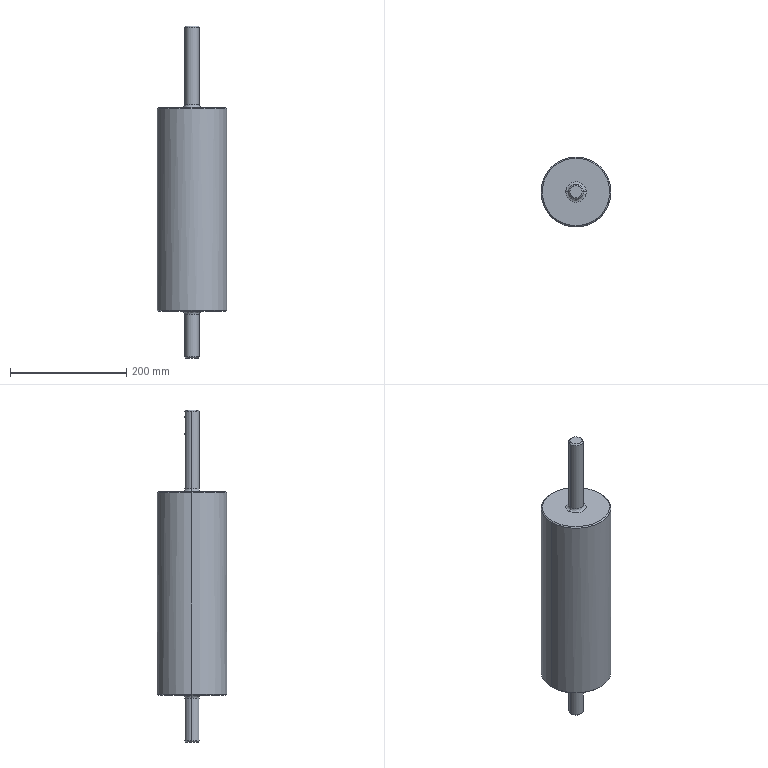Part | STEP file | Roller 1 | 1 solid | 32 faces | box 120 x 120 x 570 mm | volume 928585 mm3 | cylinder 11 | plane 9 | cone 8 | spline 4 | commonest cylinder face diameters 25 x4 8 x3 110 x2 120 x2
STEP:
#1=CARTESIAN_POINT('',(-12.5,0.,-5.));
#2=VERTEX_POINT('',#1);
#3=CARTESIAN_POINT('',(12.5,0.,-5.));
#4=VERTEX_POINT('',#3);
#5=CARTESIAN_POINT('',(0.,0.,-5.));
#6=DIRECTION('',(0.,0.,-1.));
#7=DIRECTION('',(1.,0.,0.));
#8=AXIS2_PLACEMENT_3D('',#5,#6,#7);
#9=CIRCLE('',#8,12.5);
#10=EDGE_CURVE('',#2,#4,#9,.T.);
#11=ORIENTED_EDGE('',*,*,#10,.F.);
#12=CARTESIAN_POINT('',(-17.5,0.,0.));
#13=VERTEX_POINT('',#12);
#14=CARTESIAN_POINT('',(-17.5,0.,-5.));
#15=DIRECTION('',(0.,-1.,0.));
#16=DIRECTION('',(-1.,0.,0.));
#17=AXIS2_PLACEMENT_3D('',#14,#15,#16);
#18=CIRCLE('',#17,5.);
#19=EDGE_CURVE('',#2,#13,#18,.T.);
#20=ORIENTED_EDGE('',*,*,#19,.T.);
#21=CARTESIAN_POINT('',(17.5,0.,0.));
#22=VERTEX_POINT('',#21);
#23=CARTESIAN_POINT('',(-17.5,0.,0.));
#24=CARTESIAN_POINT('',(-17.5,35.,0.));
#25=CARTESIAN_POINT('',(17.5,35.,0.));
#26=CARTESIAN_POINT('',(17.5,0.,0.));
#27=(BOUNDED_CURVE()B_SPLINE_CURVE(3,(#23,#24,#25,#26),.UNSPECIFIED.,.F.,.F.)B_SPLINE_CURVE_WITH_KNOTS((4,4),(0.,1.),.UNSPECIFIED.)CURVE()GEOMETRIC_REPRESENTATION_ITEM()RATIONAL_B_SPLINE_CURVE((1.,0.3333,0.3333,1.))REPRESENTATION_ITEM(''));
#28=EDGE_CURVE('',#13,#22,#27,.T.);
#29=ORIENTED_EDGE('',*,*,#28,.T.);
#30=CARTESIAN_POINT('',(17.5,0.,-5.));
#31=DIRECTION('',(0.,1.,0.));
#32=DIRECTION('',(1.,0.,0.));
#33=AXIS2_PLACEMENT_3D('',#30,#31,#32);
#34=CIRCLE('',#33,5.);
#35=EDGE_CURVE('',#4,#22,#34,.T.);
#36=ORIENTED_EDGE('',*,*,#35,.F.);
#37=EDGE_LOOP('',(#11,#20,#29,#36));
#38=FACE_OUTER_BOUND('',#37,.T.);
#39=CARTESIAN_POINT('',(12.5,0.,-5.));
#40=CARTESIAN_POINT('',(12.5,25.,-5.));
#41=CARTESIAN_POINT('',(-12.5,25.,-5.));
#42=CARTESIAN_POINT('',(-12.5,0.,-5.));
#43=CARTESIAN_POINT('',(12.5,0.,-2.071));
#44=CARTESIAN_POINT('',(12.5,25.,-2.071));
#45=CARTESIAN_POINT('',(-12.5,25.,-2.071));
#46=CARTESIAN_POINT('',(-12.5,0.,-2.071));
#47=CARTESIAN_POINT('',(14.571,0.,0.));
#48=CARTESIAN_POINT('',(14.571,29.142,0.));
#49=CARTESIAN_POINT('',(-14.571,29.142,0.));
#50=CARTESIAN_POINT('',(-14.571,0.,0.));
#51=CARTESIAN_POINT('',(17.5,0.,0.));
#52=CARTESIAN_POINT('',(17.5,35.,0.));
#53=CARTESIAN_POINT('',(-17.5,35.,0.));
#54=CARTESIAN_POINT('',(-17.5,0.,0.));
#55=(BOUNDED_SURFACE()B_SPLINE_SURFACE(3,3,((#39,#40,#41,#42),(#43,#44,#45,#46),(#47,#48,#49,#50),(#51,#52,#53,#54)),.UNSPECIFIED.,.F.,.F.,.F.)B_SPLINE_SURFACE_WITH_KNOTS((4,4),(4,4),(0.,1.),(0.,1.),.UNSPECIFIED.)GEOMETRIC_REPRESENTATION_ITEM()RATIONAL_B_SPLINE_SURFACE(((1.,0.3333,0.3333,1.),(0.8047,0.2682,0.2682,0.8047),(0.8047,0.2682,0.2682,0.8047),(1.,0.3333,0.3333,1.)))REPRESENTATION_ITEM('')SURFACE());
#56=ADVANCED_FACE('',(#38),#55,.F.);
#57=CARTESIAN_POINT('',(-17.5,0.,350.));
#58=VERTEX_POINT('',#57);
#59=CARTESIAN_POINT('',(17.5,0.,350.));
#60=VERTEX_POINT('',#59);
#61=CARTESIAN_POINT('',(-17.5,0.,350.));
#62=CARTESIAN_POINT('',(-17.5,0.5353,350.));
#63=CARTESIAN_POINT('',(-17.463,1.335,350.));
#64=CARTESIAN_POINT('',(-17.357,2.262,350.));
#65=CARTESIAN_POINT('',(-17.288,2.723,350.));
#66=CARTESIAN_POINT('',(-17.249,2.954,350.));
#67=CARTESIAN_POINT('',(-17.232,3.053,350.));
#68=CARTESIAN_POINT('',(-17.22,3.119,350.));
#69=CARTESIAN_POINT('',(-17.214,3.149,350.));
#70=CARTESIAN_POINT('',(-17.105,3.742,350.));
#71=CARTESIAN_POINT('',(-16.91,4.568,350.));
#72=CARTESIAN_POINT('',(-16.614,5.511,350.));
#73=CARTESIAN_POINT('',(-16.448,5.978,350.));
#74=CARTESIAN_POINT('',(-16.361,6.21,350.));
#75=CARTESIAN_POINT('',(-16.323,6.31,350.));
#76=CARTESIAN_POINT('',(-16.297,6.376,350.));
#77=CARTESIAN_POINT('',(-16.285,6.407,350.));
#78=CARTESIAN_POINT('',(-16.054,6.991,350.));
#79=CARTESIAN_POINT('',(-15.688,7.795,350.));
#80=CARTESIAN_POINT('',(-15.191,8.698,350.));
#81=CARTESIAN_POINT('',(-14.925,9.14,350.));
#82=CARTESIAN_POINT('',(-14.807,9.328,350.));
#83=CARTESIAN_POINT('',(-14.728,9.452,350.));
#84=CARTESIAN_POINT('',(-14.689,9.513,350.));
#85=CARTESIAN_POINT('',(-13.987,10.587,350.));
#86=CARTESIAN_POINT('',(-13.228,11.52,350.));
#87=CARTESIAN_POINT('',(-11.947,12.801,350.));
#88=CARTESIAN_POINT('',(-11.277,13.406,350.));
#89=CARTESIAN_POINT('',(-10.444,14.048,350.));
#90=CARTESIAN_POINT('',(-10.014,14.353,350.));
#91=CARTESIAN_POINT('',(-9.828,14.48,350.));
#92=CARTESIAN_POINT('',(-9.702,14.564,350.));
#93=CARTESIAN_POINT('',(-9.638,14.607,350.));
#94=CARTESIAN_POINT('',(-9.081,14.971,350.));
#95=CARTESIAN_POINT('',(-8.318,15.417,350.));
#96=CARTESIAN_POINT('',(-7.392,15.867,350.));
#97=CARTESIAN_POINT('',(-6.92,16.075,350.));
#98=CARTESIAN_POINT('',(-6.682,16.175,350.));
#99=CARTESIAN_POINT('',(-6.579,16.216,350.));
#100=CARTESIAN_POINT('',(-6.51,16.244,350.));
#101=CARTESIAN_POINT('',(-6.475,16.258,350.));
#102=CARTESIAN_POINT('',(-5.914,16.48,350.));
#103=CARTESIAN_POINT('',(-5.111,16.754,350.));
#104=CARTESIAN_POINT('',(-4.155,17.004,350.));
#105=CARTESIAN_POINT('',(-3.671,17.112,350.));
#106=CARTESIAN_POINT('',(-3.428,17.161,350.));
#107=CARTESIAN_POINT('',(-3.324,17.181,350.));
#108=CARTESIAN_POINT('',(-3.254,17.195,350.));
#109=CARTESIAN_POINT('',(-3.217,17.202,350.));
#110=CARTESIAN_POINT('',(-2.132,17.403,350.));
#111=CARTESIAN_POINT('',(-1.07,17.5,350.));
#112=CARTESIAN_POINT('',(0.535,17.5,350.));
#113=CARTESIAN_POINT('',(1.334,17.464,350.));
#114=CARTESIAN_POINT('',(2.261,17.357,350.));
#115=CARTESIAN_POINT('',(2.723,17.288,350.));
#116=CARTESIAN_POINT('',(2.954,17.249,350.));
#117=CARTESIAN_POINT('',(3.053,17.232,350.));
#118=CARTESIAN_POINT('',(3.119,17.22,350.));
#119=CARTESIAN_POINT('',(3.149,17.214,350.));
#120=CARTESIAN_POINT('',(3.742,17.105,350.));
#121=CARTESIAN_POINT('',(4.568,16.91,350.));
#122=CARTESIAN_POINT('',(5.511,16.614,350.));
#123=CARTESIAN_POINT('',(5.978,16.448,350.));
#124=CARTESIAN_POINT('',(6.21,16.361,350.));
#125=CARTESIAN_POINT('',(6.31,16.323,350.));
#126=CARTESIAN_POINT('',(6.376,16.297,350.));
#127=CARTESIAN_POINT('',(6.407,16.285,350.));
#128=CARTESIAN_POINT('',(6.991,16.054,350.));
#129=CARTESIAN_POINT('',(7.795,15.688,350.));
#130=CARTESIAN_POINT('',(8.698,15.191,350.));
#131=CARTESIAN_POINT('',(9.14,14.925,350.));
#132=CARTESIAN_POINT('',(9.328,14.807,350.));
#133=CARTESIAN_POINT('',(9.452,14.728,350.));
#134=CARTESIAN_POINT('',(9.513,14.689,350.));
#135=CARTESIAN_POINT('',(10.587,13.987,350.));
#136=CARTESIAN_POINT('',(11.52,13.228,350.));
#137=CARTESIAN_POINT('',(12.801,11.947,350.));
#138=CARTESIAN_POINT('',(13.406,11.277,350.));
#139=CARTESIAN_POINT('',(14.048,10.444,350.));
#140=CARTESIAN_POINT('',(14.353,10.014,350.));
#141=CARTESIAN_POINT('',(14.48,9.828,350.));
#142=CARTESIAN_POINT('',(14.564,9.702,350.));
#143=CARTESIAN_POINT('',(14.607,9.638,350.));
#144=CARTESIAN_POINT('',(14.971,9.081,350.));
#145=CARTESIAN_POINT('',(15.417,8.318,350.));
#146=CARTESIAN_POINT('',(15.867,7.392,350.));
#147=CARTESIAN_POINT('',(16.075,6.92,350.));
#148=CARTESIAN_POINT('',(16.175,6.682,350.));
#149=CARTESIAN_POINT('',(16.216,6.579,350.));
#150=CARTESIAN_POINT('',(16.244,6.51,350.));
#151=CARTESIAN_POINT('',(16.258,6.475,350.));
#152=CARTESIAN_POINT('',(16.48,5.914,350.));
#153=CARTESIAN_POINT('',(16.754,5.111,350.));
#154=CARTESIAN_POINT('',(17.004,4.155,350.));
#155=CARTESIAN_POINT('',(17.112,3.671,350.));
#156=CARTESIAN_POINT('',(17.161,3.428,350.));
#157=CARTESIAN_POINT('',(17.181,3.324,350.));
#158=CARTESIAN_POINT('',(17.195,3.254,350.));
#159=CARTESIAN_POINT('',(17.202,3.217,350.));
#160=CARTESIAN_POINT('',(17.403,2.132,350.));
#161=CARTESIAN_POINT('',(17.5,1.071,350.));
#162=CARTESIAN_POINT('',(17.5,0.,350.));
#163=B_SPLINE_CURVE_WITH_KNOTS('',3,(#61,#62,#63,#64,#65,#66,#67,#68,#69,#70,#71,#72,#73,#74,#75,#76,#77,#78,#79,#80,#81,#82,#83,#84,#85,#86,#87,#88,#89,#90,#91,#92,#93,#94,#95,#96,#97,#98,#99,#100,#101,#102,#103,#104,#105,#106,#107,#108,#109,#110,#111,#112,#113,#114,#115,#116,#117,#118,#119,#120,#121,#122,#123,#124,#125,#126,#127,#128,#129,#130,#131,#132,#133,#134,#135,#136,#137,#138,#139,#140,#141,#142,#143,#144,#145,#146,#147,#148,#149,#150,#151,#152,#153,#154,#155,#156,#157,#158,#159,#160,#161,#162),.UNSPECIFIED.,.F.,.F.,(4,1,1,1,1,2,2,1,1,1,1,2,2,1,1,1,2,2,2,1,1,1,2,2,1,1,1,1,2,2,1,1,1,1,2,2,2,1,1,1,1,2,2,1,1,1,1,2,2,1,1,1,2,2,2,1,1,1,2,2,1,1,1,1,2,2,1,1,1,1,2,2,4),(0.,0.03125,0.04688,0.05469,0.05859,0.06055,0.0625,0.09375,0.1094,0.1172,0.1211,0.123,0.125,0.1563,0.1719,0.1797,0.1836,0.1875,0.25,0.2813,0.2969,0.3047,0.3086,0.3125,0.3438,0.3594,0.3672,0.3711,0.373,0.375,0.4063,0.4219,0.4297,0.4336,0.4355,0.4375,0.5,0.5313,0.5469,0.5547,0.5586,0.5605,0.5625,0.5938,0.6094,0.6172,0.6211,0.623,0.625,0.6563,0.6719,0.6797,0.6836,0.6875,0.75,0.7813,0.7969,0.8047,0.8086,0.8125,0.8438,0.8594,0.8672,0.8711,0.873,0.875,0.9063,0.9219,0.9297,0.9336,0.9355,0.9375,1.),.UNSPECIFIED.);
#164=EDGE_CURVE('',#58,#60,#163,.T.);
#165=ORIENTED_EDGE('',*,*,#164,.F.);
#166=CARTESIAN_POINT('',(-12.5,0.,355.));
#167=VERTEX_POINT('',#166);
#168=CARTESIAN_POINT('',(-17.5,0.,355.));
#169=DIRECTION('',(0.,-1.,0.));
#170=DIRECTION('',(-1.,0.,0.));
#171=AXIS2_PLACEMENT_3D('',#168,#169,#170);
#172=CIRCLE('',#171,5.);
#173=EDGE_CURVE('',#58,#167,#172,.T.);
#174=ORIENTED_EDGE('',*,*,#173,.T.);
#175=CARTESIAN_POINT('',(12.5,0.,355.));
#176=VERTEX_POINT('',#175);
#177=CARTESIAN_POINT('',(0.,0.,355.));
#178=DIRECTION('',(0.,0.,1.));
#179=DIRECTION('',(1.,0.,0.));
#180=AXIS2_PLACEMENT_3D('',#177,#178,#179);
#181=CIRCLE('',#180,12.5);
#182=EDGE_CURVE('',#176,#167,#181,.T.);
#183=ORIENTED_EDGE('',*,*,#182,.F.);
#184=CARTESIAN_POINT('',(17.5,0.,355.));
#185=DIRECTION('',(0.,1.,0.));
#186=DIRECTION('',(1.,0.,0.));
#187=AXIS2_PLACEMENT_3D('',#184,#185,#186);
#188=CIRCLE('',#187,5.);
#189=EDGE_CURVE('',#60,#176,#188,.T.);
#190=ORIENTED_EDGE('',*,*,#189,.F.);
#191=EDGE_LOOP('',(#165,#174,#183,#190));
#192=FACE_OUTER_BOUND('',#191,.T.);
#193=CARTESIAN_POINT('',(17.5,0.,350.));
#194=CARTESIAN_POINT('',(17.5,35.,350.));
#195=CARTESIAN_POINT('',(-17.5,35.,350.));
#196=CARTESIAN_POINT('',(-17.5,0.,350.));
#197=CARTESIAN_POINT('',(14.571,0.,350.));
#198=CARTESIAN_POINT('',(14.571,29.142,350.));
#199=CARTESIAN_POINT('',(-14.571,29.142,350.));
#200=CARTESIAN_POINT('',(-14.571,0.,350.));
#201=CARTESIAN_POINT('',(12.5,0.,352.071));
#202=CARTESIAN_POINT('',(12.5,25.,352.071));
#203=CARTESIAN_POINT('',(-12.5,25.,352.071));
#204=CARTESIAN_POINT('',(-12.5,0.,352.071));
#205=CARTESIAN_POINT('',(12.5,0.,355.));
#206=CARTESIAN_POINT('',(12.5,25.,355.));
#207=CARTESIAN_POINT('',(-12.5,25.,355.));
#208=CARTESIAN_POINT('',(-12.5,0.,355.));
#209=(BOUNDED_SURFACE()B_SPLINE_SURFACE(3,3,((#193,#194,#195,#196),(#197,#198,#199,#200),(#201,#202,#203,#204),(#205,#206,#207,#208)),.UNSPECIFIED.,.F.,.F.,.F.)B_SPLINE_SURFACE_WITH_KNOTS((4,4),(4,4),(0.,1.),(0.,1.),.UNSPECIFIED.)GEOMETRIC_REPRESENTATION_ITEM()RATIONAL_B_SPLINE_SURFACE(((1.,0.3333,0.3333,1.),(0.8047,0.2682,0.2682,0.8047),(0.8047,0.2682,0.2682,0.8047),(1.,0.3333,0.3333,1.)))REPRESENTATION_ITEM('')SURFACE());
#210=ADVANCED_FACE('',(#192),#209,.F.);
#211=CARTESIAN_POINT('',(0.,60.,348.));
#212=VERTEX_POINT('',#211);
#213=CARTESIAN_POINT('',(60.,0.,348.));
#214=VERTEX_POINT('',#213);
#215=CARTESIAN_POINT('',(0.,0.,348.));
#216=DIRECTION('',(0.,0.,-1.));
#217=DIRECTION('',(-1.,0.,0.));
#218=AXIS2_PLACEMENT_3D('',#215,#216,#217);
#219=CIRCLE('',#218,60.);
#220=EDGE_CURVE('',#212,#214,#219,.T.);
#221=ORIENTED_EDGE('',*,*,#220,.T.);
#222=CARTESIAN_POINT('',(60.,0.,2.));
#223=VERTEX_POINT('',#222);
#224=CARTESIAN_POINT('',(60.,0.,350.));
#225=DIRECTION('',(0.,0.,-1.));
#226=VECTOR('',#225,1000.);
#227=LINE('',#224,#226);
#228=EDGE_CURVE('',#214,#223,#227,.T.);
#229=ORIENTED_EDGE('',*,*,#228,.T.);
#230=CARTESIAN_POINT('',(-60.,0.,2.));
#231=VERTEX_POINT('',#230);
#232=CARTESIAN_POINT('',(0.,0.,2.));
#233=DIRECTION('',(0.,0.,1.));
#234=DIRECTION('',(-1.,0.,0.));
#235=AXIS2_PLACEMENT_3D('',#232,#233,#234);
#236=CIRCLE('',#235,60.);
#237=EDGE_CURVE('',#223,#231,#236,.T.);
#238=ORIENTED_EDGE('',*,*,#237,.T.);
#239=CARTESIAN_POINT('',(-60.,0.,348.));
#240=VERTEX_POINT('',#239);
#241=CARTESIAN_POINT('',(-60.,0.,350.));
#242=DIRECTION('',(0.,0.,-1.));
#243=VECTOR('',#242,1000.);
#244=LINE('',#241,#243);
#245=EDGE_CURVE('',#240,#231,#244,.T.);
#246=ORIENTED_EDGE('',*,*,#245,.F.);
#247=CARTESIAN_POINT('',(0.,0.,348.));
#248=DIRECTION('',(0.,0.,-1.));
#249=DIRECTION('',(-1.,0.,0.));
#250=AXIS2_PLACEMENT_3D('',#247,#248,#249);
#251=CIRCLE('',#250,60.);
#252=EDGE_CURVE('',#240,#212,#251,.T.);
#253=ORIENTED_EDGE('',*,*,#252,.T.);
#254=EDGE_LOOP('',(#221,#229,#238,#246,#253));
#255=FACE_OUTER_BOUND('',#254,.T.);
#256=CARTESIAN_POINT('',(0.,0.,350.));
#257=DIRECTION('',(0.,0.,-1.));
#258=DIRECTION('',(-1.,0.,0.));
#259=AXIS2_PLACEMENT_3D('',#256,#257,#258);
#260=CYLINDRICAL_SURFACE('',#259,60.);
#261=ADVANCED_FACE('',(#255),#260,.T.);
#262=CARTESIAN_POINT('',(58.,0.,0.));
#263=VERTEX_POINT('',#262);
#264=CARTESIAN_POINT('',(-58.,0.,0.));
#265=VERTEX_POINT('',#264);
#266=CARTESIAN_POINT('',(0.,0.,0.));
#267=DIRECTION('',(0.,0.,1.));
#268=DIRECTION('',(1.,0.,0.));
#269=AXIS2_PLACEMENT_3D('',#266,#267,#268);
#270=CIRCLE('',#269,58.);
#271=EDGE_CURVE('',#263,#265,#270,.T.);
#272=ORIENTED_EDGE('',*,*,#271,.T.);
#273=CARTESIAN_POINT('',(-60.,0.,2.));
#274=DIRECTION('',(-0.7071,0.,0.7071));
#275=VECTOR('',#274,1000.);
#276=LINE('',#273,#275);
#277=EDGE_CURVE('',#265,#231,#276,.T.);
#278=ORIENTED_EDGE('',*,*,#277,.T.);
#279=ORIENTED_EDGE('',*,*,#237,.F.);
#280=CARTESIAN_POINT('',(60.,0.,2.));
#281=DIRECTION('',(0.7071,0.,0.7071));
#282=VECTOR('',#281,1000.);
#283=LINE('',#280,#282);
#284=EDGE_CURVE('',#263,#223,#283,.T.);
#285=ORIENTED_EDGE('',*,*,#284,.F.);
#286=EDGE_LOOP('',(#272,#278,#279,#285));
#287=FACE_OUTER_BOUND('',#286,.T.);
#288=CARTESIAN_POINT('',(0.,0.,2.));
#289=DIRECTION('',(0.,0.,1.));
#290=DIRECTION('',(1.,0.,0.));
#291=AXIS2_PLACEMENT_3D('',#288,#289,#290);
#292=CONICAL_SURFACE('',#291,60.,0.7854);
#293=ADVANCED_FACE('',(#287),#292,.T.);
#294=CARTESIAN_POINT('',(0.,58.,350.));
#295=VERTEX_POINT('',#294);
#296=CARTESIAN_POINT('',(0.,-58.,350.));
#297=VERTEX_POINT('',#296);
#298=CARTESIAN_POINT('',(0.,0.,350.));
#299=DIRECTION('',(0.,0.,-1.));
#300=DIRECTION('',(0.,1.,0.));
#301=AXIS2_PLACEMENT_3D('',#298,#299,#300);
#302=CIRCLE('',#301,58.);
#303=EDGE_CURVE('',#295,#297,#302,.T.);
#304=ORIENTED_EDGE('',*,*,#303,.T.);
#305=CARTESIAN_POINT('',(0.,-60.,348.));
#306=VERTEX_POINT('',#305);
#307=CARTESIAN_POINT('',(0.,-60.,348.));
#308=DIRECTION('',(0.,-0.7071,-0.7071));
#309=VECTOR('',#308,1000.);
#310=LINE('',#307,#309);
#311=EDGE_CURVE('',#297,#306,#310,.T.);
#312=ORIENTED_EDGE('',*,*,#311,.T.);
#313=CARTESIAN_POINT('',(0.,0.,348.));
#314=DIRECTION('',(0.,0.,-1.));
#315=DIRECTION('',(-1.,0.,0.));
#316=AXIS2_PLACEMENT_3D('',#313,#314,#315);
#317=CIRCLE('',#316,60.);
#318=EDGE_CURVE('',#214,#306,#317,.T.);
#319=ORIENTED_EDGE('',*,*,#318,.F.);
#320=ORIENTED_EDGE('',*,*,#220,.F.);
#321=CARTESIAN_POINT('',(0.,60.,348.));
#322=DIRECTION('',(0.,0.7071,-0.7071));
#323=VECTOR('',#322,1000.);
#324=LINE('',#321,#323);
#325=EDGE_CURVE('',#295,#212,#324,.T.);
#326=ORIENTED_EDGE('',*,*,#325,.F.);
#327=EDGE_LOOP('',(#304,#312,#319,#320,#326));
#328=FACE_OUTER_BOUND('',#327,.T.);
#329=CARTESIAN_POINT('',(0.,0.,348.));
#330=DIRECTION('',(0.,0.,-1.));
#331=DIRECTION('',(0.,1.,0.));
#332=AXIS2_PLACEMENT_3D('',#329,#330,#331);
#333=CONICAL_SURFACE('',#332,60.,0.7854);
#334=ADVANCED_FACE('',(#328),#333,.T.);
#335=CARTESIAN_POINT('',(12.5,0.,-78.));
#336=VERTEX_POINT('',#335);
#337=CARTESIAN_POINT('',(-12.5,0.,-78.));
#338=VERTEX_POINT('',#337);
#339=CARTESIAN_POINT('',(0.,0.,-78.));
#340=DIRECTION('',(0.,0.,1.));
#341=DIRECTION('',(1.,0.,0.));
#342=AXIS2_PLACEMENT_3D('',#339,#340,#341);
#343=CIRCLE('',#342,12.5);
#344=EDGE_CURVE('',#336,#338,#343,.T.);
#345=ORIENTED_EDGE('',*,*,#344,.T.);
#346=CARTESIAN_POINT('',(-12.5,0.,-80.));
#347=DIRECTION('',(0.,0.,1.));
#348=VECTOR('',#347,1000.);
#349=LINE('',#346,#348);
#350=EDGE_CURVE('',#338,#2,#349,.T.);
#351=ORIENTED_EDGE('',*,*,#350,.T.);
#352=ORIENTED_EDGE('',*,*,#10,.T.);
#353=CARTESIAN_POINT('',(12.5,0.,-80.));
#354=DIRECTION('',(0.,0.,1.));
#355=VECTOR('',#354,1000.);
#356=LINE('',#353,#355);
#357=EDGE_CURVE('',#336,#4,#356,.T.);
#358=ORIENTED_EDGE('',*,*,#357,.F.);
#359=EDGE_LOOP('',(#345,#351,#352,#358));
#360=FACE_OUTER_BOUND('',#359,.T.);
#361=CARTESIAN_POINT('',(0.,0.,-80.));
#362=DIRECTION('',(0.,0.,1.));
#363=DIRECTION('',(1.,0.,0.));
#364=AXIS2_PLACEMENT_3D('',#361,#362,#363);
#365=CYLINDRICAL_SURFACE('',#364,12.5);
#366=ADVANCED_FACE('',(#360),#365,.T.);
#367=CARTESIAN_POINT('',(4.,11.843,452.));
#368=VERTEX_POINT('',#367);
#369=CARTESIAN_POINT('',(4.,11.843,474.));
#370=VERTEX_POINT('',#369);
#371=CARTESIAN_POINT('',(4.,11.843,490.));
#372=DIRECTION('',(0.,0.,1.));
#373=VECTOR('',#372,1000.);
#374=LINE('',#371,#373);
#375=EDGE_CURVE('',#368,#370,#374,.T.);
#376=ORIENTED_EDGE('',*,*,#375,.T.);
#377=CARTESIAN_POINT('',(0.,12.5,478.));
#378=VERTEX_POINT('',#377);
#379=CARTESIAN_POINT('',(4.,11.843,474.));
#380=CARTESIAN_POINT('',(4.,11.843,474.266));
#381=CARTESIAN_POINT('',(3.974,11.852,474.527));
#382=CARTESIAN_POINT('',(3.871,11.886,475.04));
#383=CARTESIAN_POINT('',(3.794,11.911,475.295));
#384=CARTESIAN_POINT('',(3.592,11.973,475.779));
#385=CARTESIAN_POINT('',(3.47,12.01,476.007));
#386=CARTESIAN_POINT('',(3.18,12.09,476.441));
#387=CARTESIAN_POINT('',(3.012,12.133,476.644));
#388=CARTESIAN_POINT('',(2.646,12.218,477.011));
#389=CARTESIAN_POINT('',(2.446,12.26,477.176));
#390=CARTESIAN_POINT('',(2.01,12.339,477.468));
#391=CARTESIAN_POINT('',(1.78,12.375,477.591));
#392=CARTESIAN_POINT('',(1.3,12.435,477.792));
#393=CARTESIAN_POINT('',(1.047,12.459,477.87));
#394=CARTESIAN_POINT('',(0.5285,12.492,477.974));
#395=CARTESIAN_POINT('',(0.266,12.5,478.));
#396=CARTESIAN_POINT('',(0.,12.5,478.));
#397=B_SPLINE_CURVE_WITH_KNOTS('',3,(#379,#380,#381,#382,#383,#384,#385,#386,#387,#388,#389,#390,#391,#392,#393,#394,#395,#396),.UNSPECIFIED.,.F.,.F.,(4,2,2,2,2,2,2,2,4),(-0.00629,-0.005504,-0.004718,-0.003932,-0.003145,-0.002359,-0.001573,-0.0007863,0.),.UNSPECIFIED.);
#398=EDGE_CURVE('',#370,#378,#397,.T.);
#399=ORIENTED_EDGE('',*,*,#398,.T.);
#400=CARTESIAN_POINT('',(-4.,11.843,474.));
#401=VERTEX_POINT('',#400);
#402=CARTESIAN_POINT('',(0.,12.5,478.));
#403=CARTESIAN_POINT('',(-0.266,12.5,478.));
#404=CARTESIAN_POINT('',(-0.5272,12.492,477.974));
#405=CARTESIAN_POINT('',(-1.041,12.459,477.871));
#406=CARTESIAN_POINT('',(-1.296,12.435,477.793));
#407=CARTESIAN_POINT('',(-1.779,12.375,477.592));
#408=CARTESIAN_POINT('',(-2.008,12.34,477.469));
#409=CARTESIAN_POINT('',(-2.441,12.261,477.179));
#410=CARTESIAN_POINT('',(-2.645,12.218,477.012));
#411=CARTESIAN_POINT('',(-3.011,12.133,476.646));
#412=CARTESIAN_POINT('',(-3.176,12.091,476.446));
#413=CARTESIAN_POINT('',(-3.469,12.01,476.009));
#414=CARTESIAN_POINT('',(-3.592,11.973,475.78));
#415=CARTESIAN_POINT('',(-3.792,11.911,475.3));
#416=CARTESIAN_POINT('',(-3.87,11.886,475.046));
#417=CARTESIAN_POINT('',(-3.974,11.852,474.528));
#418=CARTESIAN_POINT('',(-4.,11.843,474.266));
#419=CARTESIAN_POINT('',(-4.,11.843,474.));
#420=B_SPLINE_CURVE_WITH_KNOTS('',3,(#402,#403,#404,#405,#406,#407,#408,#409,#410,#411,#412,#413,#414,#415,#416,#417,#418,#419),.UNSPECIFIED.,.F.,.F.,(4,2,2,2,2,2,2,2,4),(0.,0.0007863,0.001573,0.002359,0.003145,0.003932,0.004718,0.005504,0.00629),.UNSPECIFIED.);
#421=EDGE_CURVE('',#378,#401,#420,.T.);
#422=ORIENTED_EDGE('',*,*,#421,.T.);
#423=CARTESIAN_POINT('',(-4.,11.843,452.));
#424=VERTEX_POINT('',#423);
#425=CARTESIAN_POINT('',(-4.,11.843,490.));
#426=DIRECTION('',(0.,0.,-1.));
#427=VECTOR('',#426,1000.);
#428=LINE('',#425,#427);
#429=EDGE_CURVE('',#401,#424,#428,.T.);
#430=ORIENTED_EDGE('',*,*,#429,.T.);
#431=CARTESIAN_POINT('',(-4.,11.843,452.));
#432=CARTESIAN_POINT('',(-4.,11.843,451.734));
#433=CARTESIAN_POINT('',(-3.974,11.852,451.473));
#434=CARTESIAN_POINT('',(-3.871,11.886,450.959));
#435=CARTESIAN_POINT('',(-3.793,11.911,450.704));
#436=CARTESIAN_POINT('',(-3.592,11.973,450.221));
#437=CARTESIAN_POINT('',(-3.469,12.01,449.992));
#438=CARTESIAN_POINT('',(-3.179,12.09,449.559));
#439=CARTESIAN_POINT('',(-3.012,12.133,449.355));
#440=CARTESIAN_POINT('',(-2.646,12.218,448.989));
#441=CARTESIAN_POINT('',(-2.445,12.26,448.824));
#442=CARTESIAN_POINT('',(-2.009,12.34,448.531));
#443=CARTESIAN_POINT('',(-1.779,12.375,448.408));
#444=CARTESIAN_POINT('',(-1.299,12.435,448.208));
#445=CARTESIAN_POINT('',(-1.045,12.459,448.13));
#446=CARTESIAN_POINT('',(-0.5276,12.492,448.026));
#447=CARTESIAN_POINT('',(-0.2669,12.5,448.));
#448=CARTESIAN_POINT('',(0.2587,12.5,448.));
#449=CARTESIAN_POINT('',(0.5256,12.492,448.026));
#450=CARTESIAN_POINT('',(1.04,12.459,448.129));
#451=CARTESIAN_POINT('',(1.29,12.436,448.205));
#452=CARTESIAN_POINT('',(1.777,12.375,448.407));
#453=CARTESIAN_POINT('',(2.008,12.34,448.531));
#454=CARTESIAN_POINT('',(2.44,12.262,448.82));
#455=CARTESIAN_POINT('',(2.643,12.219,448.987));
#456=CARTESIAN_POINT('',(3.012,12.133,449.355));
#457=CARTESIAN_POINT('',(3.176,12.091,449.555));
#458=CARTESIAN_POINT('',(3.466,12.011,449.987));
#459=CARTESIAN_POINT('',(3.592,11.973,450.22));
#460=CARTESIAN_POINT('',(3.792,11.911,450.702));
#461=CARTESIAN_POINT('',(3.869,11.886,450.951));
#462=CARTESIAN_POINT('',(3.973,11.852,451.468));
#463=CARTESIAN_POINT('',(4.,11.843,451.734));
#464=CARTESIAN_POINT('',(4.,11.843,452.));
#465=B_SPLINE_CURVE_WITH_KNOTS('',3,(#431,#432,#433,#434,#435,#436,#437,#438,#439,#440,#441,#442,#443,#444,#445,#446,#447,#448,#449,#450,#451,#452,#453,#454,#455,#456,#457,#458,#459,#460,#461,#462,#463,#464),.UNSPECIFIED.,.F.,.F.,(4,2,2,2,2,2,2,2,2,2,2,2,2,2,2,2,4),(0.,0.0007865,0.001573,0.00236,0.003146,0.003933,0.004719,0.005506,0.006292,0.007079,0.007865,0.008652,0.009438,0.01022,0.01101,0.0118,0.01258),.UNSPECIFIED.);
#466=EDGE_CURVE('',#424,#368,#465,.T.);
#467=ORIENTED_EDGE('',*,*,#466,.T.);
#468=EDGE_LOOP('',(#376,#399,#422,#430,#467));
#469=FACE_BOUND('',#468,.T.);
#470=CARTESIAN_POINT('',(-12.5,0.,488.));
#471=VERTEX_POINT('',#470);
#472=CARTESIAN_POINT('',(12.5,0.,488.));
#473=VERTEX_POINT('',#472);
#474=CARTESIAN_POINT('',(0.,0.,488.));
#475=DIRECTION('',(0.,0.,-1.));
#476=DIRECTION('',(-1.,0.,0.));
#477=AXIS2_PLACEMENT_3D('',#474,#475,#476);
#478=CIRCLE('',#477,12.5);
#479=EDGE_CURVE('',#471,#473,#478,.T.);
#480=ORIENTED_EDGE('',*,*,#479,.T.);
#481=CARTESIAN_POINT('',(12.5,0.,490.));
#482=DIRECTION('',(0.,0.,-1.));
#483=VECTOR('',#482,1000.);
#484=LINE('',#481,#483);
#485=EDGE_CURVE('',#473,#176,#484,.T.);
#486=ORIENTED_EDGE('',*,*,#485,.T.);
#487=ORIENTED_EDGE('',*,*,#182,.T.);
#488=CARTESIAN_POINT('',(-12.5,0.,490.));
#489=DIRECTION('',(0.,0.,-1.));
#490=VECTOR('',#489,1000.);
#491=LINE('',#488,#490);
#492=EDGE_CURVE('',#471,#167,#491,.T.);
#493=ORIENTED_EDGE('',*,*,#492,.F.);
#494=EDGE_LOOP('',(#480,#486,#487,#493));
#495=FACE_OUTER_BOUND('',#494,.T.);
#496=CARTESIAN_POINT('',(0.,0.,490.));
#497=DIRECTION('',(0.,0.,-1.));
#498=DIRECTION('',(-1.,0.,0.));
#499=AXIS2_PLACEMENT_3D('',#496,#497,#498);
#500=CYLINDRICAL_SURFACE('',#499,12.5);
#501=ADVANCED_FACE('',(#469,#495),#500,.T.);
#502=CARTESIAN_POINT('',(10.5,0.,-80.));
#503=VERTEX_POINT('',#502);
#504=CARTESIAN_POINT('',(-10.5,0.,-80.));
#505=VERTEX_POINT('',#504);
#506=CARTESIAN_POINT('',(0.,0.,-80.));
#507=DIRECTION('',(0.,0.,1.));
#508=DIRECTION('',(1.,0.,0.));
#509=AXIS2_PLACEMENT_3D('',#506,#507,#508);
#510=CIRCLE('',#509,10.5);
#511=EDGE_CURVE('',#503,#505,#510,.T.);
#512=ORIENTED_EDGE('',*,*,#511,.T.);
#513=CARTESIAN_POINT('',(-12.5,0.,-78.));
#514=DIRECTION('',(-0.7071,0.,0.7071));
#515=VECTOR('',#514,1000.);
#516=LINE('',#513,#515);
#517=EDGE_CURVE('',#505,#338,#516,.T.);
#518=ORIENTED_EDGE('',*,*,#517,.T.);
#519=ORIENTED_EDGE('',*,*,#344,.F.);
#520=CARTESIAN_POINT('',(12.5,0.,-78.));
#521=DIRECTION('',(0.7071,0.,0.7071));
#522=VECTOR('',#521,1000.);
#523=LINE('',#520,#522);
#524=EDGE_CURVE('',#503,#336,#523,.T.);
#525=ORIENTED_EDGE('',*,*,#524,.F.);
#526=EDGE_LOOP('',(#512,#518,#519,#525));
#527=FACE_OUTER_BOUND('',#526,.T.);
#528=CARTESIAN_POINT('',(0.,0.,-78.));
#529=DIRECTION('',(0.,0.,1.));
#530=DIRECTION('',(1.,0.,0.));
#531=AXIS2_PLACEMENT_3D('',#528,#529,#530);
#532=CONICAL_SURFACE('',#531,12.5,0.7854);
#533=ADVANCED_FACE('',(#527),#532,.T.);
#534=CARTESIAN_POINT('',(-10.5,0.,490.));
#535=VERTEX_POINT('',#534);
#536=CARTESIAN_POINT('',(10.5,0.,490.));
#537=VERTEX_POINT('',#536);
#538=CARTESIAN_POINT('',(0.,0.,490.));
#539=DIRECTION('',(0.,0.,-1.));
#540=DIRECTION('',(-1.,0.,0.));
#541=AXIS2_PLACEMENT_3D('',#538,#539,#540);
#542=CIRCLE('',#541,10.5);
#543=EDGE_CURVE('',#535,#537,#542,.T.);
#544=ORIENTED_EDGE('',*,*,#543,.T.);
#545=CARTESIAN_POINT('',(12.5,0.,488.));
#546=DIRECTION('',(0.7071,0.,-0.7071));
#547=VECTOR('',#546,1000.);
#548=LINE('',#545,#547);
#549=EDGE_CURVE('',#537,#473,#548,.T.);
#550=ORIENTED_EDGE('',*,*,#549,.T.);
#551=ORIENTED_EDGE('',*,*,#479,.F.);
#552=CARTESIAN_POINT('',(-12.5,0.,488.));
#553=DIRECTION('',(-0.7071,0.,-0.7071));
#554=VECTOR('',#553,1000.);
#555=LINE('',#552,#554);
#556=EDGE_CURVE('',#535,#471,#555,.T.);
#557=ORIENTED_EDGE('',*,*,#556,.F.);
#558=EDGE_LOOP('',(#544,#550,#551,#557));
#559=FACE_OUTER_BOUND('',#558,.T.);
#560=CARTESIAN_POINT('',(0.,0.,488.));
#561=DIRECTION('',(0.,0.,-1.));
#562=DIRECTION('',(-1.,0.,0.));
#563=AXIS2_PLACEMENT_3D('',#560,#561,#562);
#564=CONICAL_SURFACE('',#563,12.5,0.7854);
#565=ADVANCED_FACE('',(#559),#564,.T.);
#566=CARTESIAN_POINT('',(0.,8.5,478.));
#567=VERTEX_POINT('',#566);
#568=CARTESIAN_POINT('',(4.,8.5,474.));
#569=VERTEX_POINT('',#568);
#570=CARTESIAN_POINT('',(0.,8.5,474.));
#571=DIRECTION('',(0.,1.,0.));
#572=DIRECTION('',(0.,0.,1.));
#573=AXIS2_PLACEMENT_3D('',#570,#571,#572);
#574=CIRCLE('',#573,4.);
#575=EDGE_CURVE('',#567,#569,#574,.T.);
#576=ORIENTED_EDGE('',*,*,#575,.F.);
#577=CARTESIAN_POINT('',(0.,8.5,478.));
#578=DIRECTION('',(0.,1.,0.));
#579=VECTOR('',#578,1000.);
#580=LINE('',#577,#579);
#581=EDGE_CURVE('',#567,#378,#580,.T.);
#582=ORIENTED_EDGE('',*,*,#581,.T.);
#583=ORIENTED_EDGE('',*,*,#398,.F.);
#584=CARTESIAN_POINT('',(4.,8.5,474.));
#585=DIRECTION('',(0.,1.,0.));
#586=VECTOR('',#585,1000.);
#587=LINE('',#584,#586);
#588=EDGE_CURVE('',#569,#370,#587,.T.);
#589=ORIENTED_EDGE('',*,*,#588,.F.);
#590=EDGE_LOOP('',(#576,#582,#583,#589));
#591=FACE_OUTER_BOUND('',#590,.T.);
#592=CARTESIAN_POINT('',(0.,8.5,474.));
#593=DIRECTION('',(0.,1.,0.));
#594=DIRECTION('',(0.,0.,1.));
#595=AXIS2_PLACEMENT_3D('',#592,#593,#594);
#596=CYLINDRICAL_SURFACE('',#595,4.);
#597=ADVANCED_FACE('',(#591),#596,.F.);
#598=CARTESIAN_POINT('',(4.,8.5,452.));
#599=VERTEX_POINT('',#598);
#600=CARTESIAN_POINT('',(-4.,8.5,452.));
#601=VERTEX_POINT('',#600);
#602=CARTESIAN_POINT('',(0.,8.5,452.));
#603=DIRECTION('',(0.,1.,0.));
#604=DIRECTION('',(0.,0.,1.));
#605=AXIS2_PLACEMENT_3D('',#602,#603,#604);
#606=CIRCLE('',#605,4.);
#607=EDGE_CURVE('',#599,#601,#606,.T.);
#608=ORIENTED_EDGE('',*,*,#607,.T.);
#609=CARTESIAN_POINT('',(-4.,8.5,474.));
#610=VERTEX_POINT('',#609);
#611=CARTESIAN_POINT('',(-4.,8.5,474.));
#612=DIRECTION('',(0.,0.,1.));
#613=VECTOR('',#612,1000.);
#614=LINE('',#611,#613);
#615=EDGE_CURVE('',#601,#610,#614,.T.);
#616=ORIENTED_EDGE('',*,*,#615,.T.);
#617=CARTESIAN_POINT('',(0.,8.5,474.));
#618=DIRECTION('',(0.,1.,0.));
#619=DIRECTION('',(0.,0.,1.));
#620=AXIS2_PLACEMENT_3D('',#617,#618,#619);
#621=CIRCLE('',#620,4.);
#622=EDGE_CURVE('',#610,#567,#621,.T.);
#623=ORIENTED_EDGE('',*,*,#622,.T.);
#624=ORIENTED_EDGE('',*,*,#575,.T.);
#625=CARTESIAN_POINT('',(4.,8.5,474.));
#626=DIRECTION('',(0.,0.,-1.));
#627=VECTOR('',#626,1000.);
#628=LINE('',#625,#627);
#629=EDGE_CURVE('',#569,#599,#628,.T.);
#630=ORIENTED_EDGE('',*,*,#629,.T.);
#631=EDGE_LOOP('',(#608,#616,#623,#624,#630));
#632=FACE_OUTER_BOUND('',#631,.T.);
#633=CARTESIAN_POINT('',(0.,8.5,474.));
#634=DIRECTION('',(0.,1.,0.));
#635=DIRECTION('',(0.,0.,1.));
#636=AXIS2_PLACEMENT_3D('',#633,#634,#635);
#637=PLANE('',#636);
#638=ADVANCED_FACE('',(#632),#637,.T.);
#639=ORIENTED_EDGE('',*,*,#543,.F.);
#640=CARTESIAN_POINT('',(0.,0.,490.));
#641=DIRECTION('',(0.,0.,-1.));
#642=DIRECTION('',(-1.,0.,0.));
#643=AXIS2_PLACEMENT_3D('',#640,#641,#642);
#644=CIRCLE('',#643,10.5);
#645=EDGE_CURVE('',#537,#535,#644,.T.);
#646=ORIENTED_EDGE('',*,*,#645,.F.);
#647=EDGE_LOOP('',(#639,#646));
#648=FACE_OUTER_BOUND('',#647,.T.);
#649=CARTESIAN_POINT('',(0.,0.,490.));
#650=DIRECTION('',(0.,0.,1.));
#651=DIRECTION('',(1.,0.,0.));
#652=AXIS2_PLACEMENT_3D('',#649,#650,#651);
#653=PLANE('',#652);
#654=ADVANCED_FACE('',(#648),#653,.T.);
#655=ORIENTED_EDGE('',*,*,#511,.F.);
#656=CARTESIAN_POINT('',(0.,0.,-80.));
#657=DIRECTION('',(0.,0.,1.));
#658=DIRECTION('',(1.,0.,0.));
#659=AXIS2_PLACEMENT_3D('',#656,#657,#658);
#660=CIRCLE('',#659,10.5);
#661=EDGE_CURVE('',#505,#503,#660,.T.);
#662=ORIENTED_EDGE('',*,*,#661,.F.);
#663=EDGE_LOOP('',(#655,#662));
#664=FACE_OUTER_BOUND('',#663,.T.);
#665=CARTESIAN_POINT('',(0.,0.,-80.));
#666=DIRECTION('',(0.,0.,-1.));
#667=DIRECTION('',(-1.,0.,0.));
#668=AXIS2_PLACEMENT_3D('',#665,#666,#667);
#669=PLANE('',#668);
#670=ADVANCED_FACE('',(#664),#669,.T.);
#671=ORIENTED_EDGE('',*,*,#615,.F.);
#672=CARTESIAN_POINT('',(-4.,8.5,452.));
#673=DIRECTION('',(0.,1.,0.));
#674=VECTOR('',#673,1000.);
#675=LINE('',#672,#674);
#676=EDGE_CURVE('',#601,#424,#675,.T.);
#677=ORIENTED_EDGE('',*,*,#676,.T.);
#678=ORIENTED_EDGE('',*,*,#429,.F.);
#679=CARTESIAN_POINT('',(-4.,8.5,474.));
#680=DIRECTION('',(0.,-1.,0.));
#681=VECTOR('',#680,1000.);
#682=LINE('',#679,#681);
#683=EDGE_CURVE('',#401,#610,#682,.T.);
#684=ORIENTED_EDGE('',*,*,#683,.T.);
#685=EDGE_LOOP('',(#671,#677,#678,#684));
#686=FACE_OUTER_BOUND('',#685,.T.);
#687=CARTESIAN_POINT('',(-4.,8.5,474.));
#688=DIRECTION('',(-1.,0.,0.));
#689=DIRECTION('',(0.,0.,1.));
#690=AXIS2_PLACEMENT_3D('',#687,#688,#689);
#691=PLANE('',#690);
#692=ADVANCED_FACE('',(#686),#691,.F.);
#693=ORIENTED_EDGE('',*,*,#607,.F.);
#694=CARTESIAN_POINT('',(4.,8.5,452.));
#695=DIRECTION('',(0.,1.,0.));
#696=VECTOR('',#695,1000.);
#697=LINE('',#694,#696);
#698=EDGE_CURVE('',#599,#368,#697,.T.);
#699=ORIENTED_EDGE('',*,*,#698,.T.);
#700=ORIENTED_EDGE('',*,*,#466,.F.);
#701=ORIENTED_EDGE('',*,*,#676,.F.);
#702=EDGE_LOOP('',(#693,#699,#700,#701));
#703=FACE_OUTER_BOUND('',#702,.T.);
#704=CARTESIAN_POINT('',(0.,8.5,452.));
#705=DIRECTION('',(0.,1.,0.));
#706=DIRECTION('',(0.,0.,1.));
#707=AXIS2_PLACEMENT_3D('',#704,#705,#706);
#708=CYLINDRICAL_SURFACE('',#707,4.);
#709=ADVANCED_FACE('',(#703),#708,.F.);
#710=ORIENTED_EDGE('',*,*,#629,.F.);
#711=ORIENTED_EDGE('',*,*,#588,.T.);
#712=ORIENTED_EDGE('',*,*,#375,.F.);
#713=ORIENTED_EDGE('',*,*,#698,.F.);
#714=EDGE_LOOP('',(#710,#711,#712,#713));
#715=FACE_OUTER_BOUND('',#714,.T.);
#716=CARTESIAN_POINT('',(4.,8.5,474.));
#717=DIRECTION('',(1.,0.,0.));
#718=DIRECTION('',(0.,0.,-1.));
#719=AXIS2_PLACEMENT_3D('',#716,#717,#718);
#720=PLANE('',#719);
#721=ADVANCED_FACE('',(#715),#720,.F.);
#722=ORIENTED_EDGE('',*,*,#581,.F.);
#723=ORIENTED_EDGE('',*,*,#622,.F.);
#724=ORIENTED_EDGE('',*,*,#683,.F.);
#725=ORIENTED_EDGE('',*,*,#421,.F.);
#726=EDGE_LOOP('',(#722,#723,#724,#725));
#727=FACE_OUTER_BOUND('',#726,.T.);
#728=CARTESIAN_POINT('',(0.,8.5,474.));
#729=DIRECTION('',(0.,1.,0.));
#730=DIRECTION('',(0.,0.,1.));
#731=AXIS2_PLACEMENT_3D('',#728,#729,#730);
#732=CYLINDRICAL_SURFACE('',#731,4.);
#733=ADVANCED_FACE('',(#727),#732,.F.);
#734=ORIENTED_EDGE('',*,*,#549,.F.);
#735=ORIENTED_EDGE('',*,*,#645,.T.);
#736=ORIENTED_EDGE('',*,*,#556,.T.);
#737=CARTESIAN_POINT('',(0.,0.,488.));
#738=DIRECTION('',(0.,0.,-1.));
#739=DIRECTION('',(-1.,0.,0.));
#740=AXIS2_PLACEMENT_3D('',#737,#738,#739);
#741=CIRCLE('',#740,12.5);
#742=EDGE_CURVE('',#473,#471,#741,.T.);
#743=ORIENTED_EDGE('',*,*,#742,.F.);
#744=EDGE_LOOP('',(#734,#735,#736,#743));
#745=FACE_OUTER_BOUND('',#744,.T.);
#746=CARTESIAN_POINT('',(0.,0.,488.));
#747=DIRECTION('',(0.,0.,-1.));
#748=DIRECTION('',(-1.,0.,0.));
#749=AXIS2_PLACEMENT_3D('',#746,#747,#748);
#750=CONICAL_SURFACE('',#749,12.5,0.7854);
#751=ADVANCED_FACE('',(#745),#750,.T.);
#752=ORIENTED_EDGE('',*,*,#517,.F.);
#753=ORIENTED_EDGE('',*,*,#661,.T.);
#754=ORIENTED_EDGE('',*,*,#524,.T.);
#755=CARTESIAN_POINT('',(0.,0.,-78.));
#756=DIRECTION('',(0.,0.,1.));
#757=DIRECTION('',(1.,0.,0.));
#758=AXIS2_PLACEMENT_3D('',#755,#756,#757);
#759=CIRCLE('',#758,12.5);
#760=EDGE_CURVE('',#338,#336,#759,.T.);
#761=ORIENTED_EDGE('',*,*,#760,.F.);
#762=EDGE_LOOP('',(#752,#753,#754,#761));
#763=FACE_OUTER_BOUND('',#762,.T.);
#764=CARTESIAN_POINT('',(0.,0.,-78.));
#765=DIRECTION('',(0.,0.,1.));
#766=DIRECTION('',(1.,0.,0.));
#767=AXIS2_PLACEMENT_3D('',#764,#765,#766);
#768=CONICAL_SURFACE('',#767,12.5,0.7854);
#769=ADVANCED_FACE('',(#763),#768,.T.);
#770=ORIENTED_EDGE('',*,*,#485,.F.);
#771=ORIENTED_EDGE('',*,*,#742,.T.);
#772=ORIENTED_EDGE('',*,*,#492,.T.);
#773=CARTESIAN_POINT('',(0.,0.,355.));
#774=DIRECTION('',(0.,0.,1.));
#775=DIRECTION('',(1.,0.,0.));
#776=AXIS2_PLACEMENT_3D('',#773,#774,#775);
#777=CIRCLE('',#776,12.5);
#778=EDGE_CURVE('',#167,#176,#777,.T.);
#779=ORIENTED_EDGE('',*,*,#778,.T.);
#780=EDGE_LOOP('',(#770,#771,#772,#779));
#781=FACE_OUTER_BOUND('',#780,.T.);
#782=CARTESIAN_POINT('',(0.,0.,490.));
#783=DIRECTION('',(0.,0.,-1.));
#784=DIRECTION('',(-1.,0.,0.));
#785=AXIS2_PLACEMENT_3D('',#782,#783,#784);
#786=CYLINDRICAL_SURFACE('',#785,12.5);
#787=ADVANCED_FACE('',(#781),#786,.T.);
#788=ORIENTED_EDGE('',*,*,#350,.F.);
#789=ORIENTED_EDGE('',*,*,#760,.T.);
#790=ORIENTED_EDGE('',*,*,#357,.T.);
#791=CARTESIAN_POINT('',(0.,0.,-5.));
#792=DIRECTION('',(0.,0.,-1.));
#793=DIRECTION('',(1.,0.,0.));
#794=AXIS2_PLACEMENT_3D('',#791,#792,#793);
#795=CIRCLE('',#794,12.5);
#796=EDGE_CURVE('',#4,#2,#795,.T.);
#797=ORIENTED_EDGE('',*,*,#796,.T.);
#798=EDGE_LOOP('',(#788,#789,#790,#797));
#799=FACE_OUTER_BOUND('',#798,.T.);
#800=CARTESIAN_POINT('',(0.,0.,-80.));
#801=DIRECTION('',(0.,0.,1.));
#802=DIRECTION('',(1.,0.,0.));
#803=AXIS2_PLACEMENT_3D('',#800,#801,#802);
#804=CYLINDRICAL_SURFACE('',#803,12.5);
#805=ADVANCED_FACE('',(#799),#804,.T.);
#806=ORIENTED_EDGE('',*,*,#173,.F.);
#807=CARTESIAN_POINT('',(17.5,0.,350.));
#808=CARTESIAN_POINT('',(17.5,-0.5353,350.));
#809=CARTESIAN_POINT('',(17.463,-1.335,350.));
#810=CARTESIAN_POINT('',(17.357,-2.262,350.));
#811=CARTESIAN_POINT('',(17.288,-2.723,350.));
#812=CARTESIAN_POINT('',(17.249,-2.954,350.));
#813=CARTESIAN_POINT('',(17.232,-3.053,350.));
#814=CARTESIAN_POINT('',(17.22,-3.119,350.));
#815=CARTESIAN_POINT('',(17.214,-3.149,350.));
#816=CARTESIAN_POINT('',(17.105,-3.742,350.));
#817=CARTESIAN_POINT('',(16.91,-4.568,350.));
#818=CARTESIAN_POINT('',(16.614,-5.511,350.));
#819=CARTESIAN_POINT('',(16.448,-5.978,350.));
#820=CARTESIAN_POINT('',(16.361,-6.21,350.));
#821=CARTESIAN_POINT('',(16.323,-6.31,350.));
#822=CARTESIAN_POINT('',(16.297,-6.376,350.));
#823=CARTESIAN_POINT('',(16.285,-6.407,350.));
#824=CARTESIAN_POINT('',(16.054,-6.991,350.));
#825=CARTESIAN_POINT('',(15.688,-7.795,350.));
#826=CARTESIAN_POINT('',(15.191,-8.698,350.));
#827=CARTESIAN_POINT('',(14.925,-9.14,350.));
#828=CARTESIAN_POINT('',(14.807,-9.328,350.));
#829=CARTESIAN_POINT('',(14.728,-9.452,350.));
#830=CARTESIAN_POINT('',(14.689,-9.513,350.));
#831=CARTESIAN_POINT('',(13.987,-10.587,350.));
#832=CARTESIAN_POINT('',(13.228,-11.52,350.));
#833=CARTESIAN_POINT('',(11.947,-12.801,350.));
#834=CARTESIAN_POINT('',(11.277,-13.406,350.));
#835=CARTESIAN_POINT('',(10.444,-14.048,350.));
#836=CARTESIAN_POINT('',(10.014,-14.353,350.));
#837=CARTESIAN_POINT('',(9.828,-14.48,350.));
#838=CARTESIAN_POINT('',(9.702,-14.564,350.));
#839=CARTESIAN_POINT('',(9.638,-14.607,350.));
#840=CARTESIAN_POINT('',(9.081,-14.971,350.));
#841=CARTESIAN_POINT('',(8.318,-15.417,350.));
#842=CARTESIAN_POINT('',(7.392,-15.867,350.));
#843=CARTESIAN_POINT('',(6.92,-16.075,350.));
#844=CARTESIAN_POINT('',(6.682,-16.175,350.));
#845=CARTESIAN_POINT('',(6.579,-16.216,350.));
#846=CARTESIAN_POINT('',(6.51,-16.244,350.));
#847=CARTESIAN_POINT('',(6.475,-16.258,350.));
#848=CARTESIAN_POINT('',(5.914,-16.48,350.));
#849=CARTESIAN_POINT('',(5.111,-16.754,350.));
#850=CARTESIAN_POINT('',(4.155,-17.004,350.));
#851=CARTESIAN_POINT('',(3.671,-17.112,350.));
#852=CARTESIAN_POINT('',(3.428,-17.161,350.));
#853=CARTESIAN_POINT('',(3.324,-17.181,350.));
#854=CARTESIAN_POINT('',(3.254,-17.195,350.));
#855=CARTESIAN_POINT('',(3.217,-17.202,350.));
#856=CARTESIAN_POINT('',(2.132,-17.403,350.));
#857=CARTESIAN_POINT('',(1.07,-17.5,350.));
#858=CARTESIAN_POINT('',(-0.535,-17.5,350.));
#859=CARTESIAN_POINT('',(-1.334,-17.464,350.));
#860=CARTESIAN_POINT('',(-2.261,-17.357,350.));
#861=CARTESIAN_POINT('',(-2.723,-17.288,350.));
#862=CARTESIAN_POINT('',(-2.954,-17.249,350.));
#863=CARTESIAN_POINT('',(-3.053,-17.232,350.));
#864=CARTESIAN_POINT('',(-3.119,-17.22,350.));
#865=CARTESIAN_POINT('',(-3.149,-17.214,350.));
#866=CARTESIAN_POINT('',(-3.742,-17.105,350.));
#867=CARTESIAN_POINT('',(-4.568,-16.91,350.));
#868=CARTESIAN_POINT('',(-5.511,-16.614,350.));
#869=CARTESIAN_POINT('',(-5.978,-16.448,350.));
#870=CARTESIAN_POINT('',(-6.21,-16.361,350.));
#871=CARTESIAN_POINT('',(-6.31,-16.323,350.));
#872=CARTESIAN_POINT('',(-6.376,-16.297,350.));
#873=CARTESIAN_POINT('',(-6.407,-16.285,350.));
#874=CARTESIAN_POINT('',(-6.991,-16.054,350.));
#875=CARTESIAN_POINT('',(-7.795,-15.688,350.));
#876=CARTESIAN_POINT('',(-8.698,-15.191,350.));
#877=CARTESIAN_POINT('',(-9.14,-14.925,350.));
#878=CARTESIAN_POINT('',(-9.328,-14.807,350.));
#879=CARTESIAN_POINT('',(-9.452,-14.728,350.));
#880=CARTESIAN_POINT('',(-9.513,-14.689,350.));
#881=CARTESIAN_POINT('',(-10.587,-13.987,350.));
#882=CARTESIAN_POINT('',(-11.52,-13.228,350.));
#883=CARTESIAN_POINT('',(-12.801,-11.947,350.));
#884=CARTESIAN_POINT('',(-13.406,-11.277,350.));
#885=CARTESIAN_POINT('',(-14.048,-10.444,350.));
#886=CARTESIAN_POINT('',(-14.353,-10.014,350.));
#887=CARTESIAN_POINT('',(-14.48,-9.828,350.));
#888=CARTESIAN_POINT('',(-14.564,-9.702,350.));
#889=CARTESIAN_POINT('',(-14.607,-9.638,350.));
#890=CARTESIAN_POINT('',(-14.971,-9.081,350.));
#891=CARTESIAN_POINT('',(-15.417,-8.318,350.));
#892=CARTESIAN_POINT('',(-15.867,-7.392,350.));
#893=CARTESIAN_POINT('',(-16.075,-6.92,350.));
#894=CARTESIAN_POINT('',(-16.175,-6.682,350.));
#895=CARTESIAN_POINT('',(-16.216,-6.579,350.));
#896=CARTESIAN_POINT('',(-16.244,-6.51,350.));
#897=CARTESIAN_POINT('',(-16.258,-6.475,350.));
#898=CARTESIAN_POINT('',(-16.48,-5.914,350.));
#899=CARTESIAN_POINT('',(-16.754,-5.111,350.));
#900=CARTESIAN_POINT('',(-17.004,-4.155,350.));
#901=CARTESIAN_POINT('',(-17.112,-3.671,350.));
#902=CARTESIAN_POINT('',(-17.161,-3.428,350.));
#903=CARTESIAN_POINT('',(-17.181,-3.324,350.));
#904=CARTESIAN_POINT('',(-17.195,-3.254,350.));
#905=CARTESIAN_POINT('',(-17.202,-3.217,350.));
#906=CARTESIAN_POINT('',(-17.403,-2.132,350.));
#907=CARTESIAN_POINT('',(-17.5,-1.071,350.));
#908=CARTESIAN_POINT('',(-17.5,0.,350.));
#909=B_SPLINE_CURVE_WITH_KNOTS('',3,(#807,#808,#809,#810,#811,#812,#813,#814,#815,#816,#817,#818,#819,#820,#821,#822,#823,#824,#825,#826,#827,#828,#829,#830,#831,#832,#833,#834,#835,#836,#837,#838,#839,#840,#841,#842,#843,#844,#845,#846,#847,#848,#849,#850,#851,#852,#853,#854,#855,#856,#857,#858,#859,#860,#861,#862,#863,#864,#865,#866,#867,#868,#869,#870,#871,#872,#873,#874,#875,#876,#877,#878,#879,#880,#881,#882,#883,#884,#885,#886,#887,#888,#889,#890,#891,#892,#893,#894,#895,#896,#897,#898,#899,#900,#901,#902,#903,#904,#905,#906,#907,#908),.UNSPECIFIED.,.F.,.F.,(4,1,1,1,1,2,2,1,1,1,1,2,2,1,1,1,2,2,2,1,1,1,2,2,1,1,1,1,2,2,1,1,1,1,2,2,2,1,1,1,1,2,2,1,1,1,1,2,2,1,1,1,2,2,2,1,1,1,2,2,1,1,1,1,2,2,1,1,1,1,2,2,4),(0.,0.03125,0.04687,0.05469,0.05859,0.06055,0.0625,0.09375,0.1094,0.1172,0.1211,0.123,0.125,0.1562,0.1719,0.1797,0.1836,0.1875,0.25,0.2812,0.2969,0.3047,0.3086,0.3125,0.3437,0.3594,0.3672,0.3711,0.373,0.375,0.4062,0.4219,0.4297,0.4336,0.4355,0.4375,0.5,0.5312,0.5469,0.5547,0.5586,0.5605,0.5625,0.5938,0.6094,0.6172,0.6211,0.623,0.625,0.6563,0.6719,0.6797,0.6836,0.6875,0.75,0.7813,0.7969,0.8047,0.8086,0.8125,0.8438,0.8594,0.8672,0.8711,0.873,0.875,0.9063,0.9219,0.9297,0.9336,0.9355,0.9375,1.),.UNSPECIFIED.);
#910=EDGE_CURVE('',#60,#58,#909,.T.);
#911=ORIENTED_EDGE('',*,*,#910,.F.);
#912=ORIENTED_EDGE('',*,*,#189,.T.);
#913=ORIENTED_EDGE('',*,*,#778,.F.);
#914=EDGE_LOOP('',(#806,#911,#912,#913));
#915=FACE_OUTER_BOUND('',#914,.T.);
#916=CARTESIAN_POINT('',(-17.5,0.,350.));
#917=CARTESIAN_POINT('',(-17.5,-35.,350.));
#918=CARTESIAN_POINT('',(17.5,-35.,350.));
#919=CARTESIAN_POINT('',(17.5,0.,350.));
#920=CARTESIAN_POINT('',(-14.571,0.,350.));
#921=CARTESIAN_POINT('',(-14.571,-29.142,350.));
#922=CARTESIAN_POINT('',(14.571,-29.142,350.));
#923=CARTESIAN_POINT('',(14.571,0.,350.));
#924=CARTESIAN_POINT('',(-12.5,0.,352.071));
#925=CARTESIAN_POINT('',(-12.5,-25.,352.071));
#926=CARTESIAN_POINT('',(12.5,-25.,352.071));
#927=CARTESIAN_POINT('',(12.5,0.,352.071));
#928=CARTESIAN_POINT('',(-12.5,0.,355.));
#929=CARTESIAN_POINT('',(-12.5,-25.,355.));
#930=CARTESIAN_POINT('',(12.5,-25.,355.));
#931=CARTESIAN_POINT('',(12.5,0.,355.));
#932=(BOUNDED_SURFACE()B_SPLINE_SURFACE(3,3,((#916,#917,#918,#919),(#920,#921,#922,#923),(#924,#925,#926,#927),(#928,#929,#930,#931)),.UNSPECIFIED.,.F.,.F.,.F.)B_SPLINE_SURFACE_WITH_KNOTS((4,4),(4,4),(0.,1.),(0.,1.),.UNSPECIFIED.)GEOMETRIC_REPRESENTATION_ITEM()RATIONAL_B_SPLINE_SURFACE(((1.,0.3333,0.3333,1.),(0.8047,0.2682,0.2682,0.8047),(0.8047,0.2682,0.2682,0.8047),(1.,0.3333,0.3333,1.)))REPRESENTATION_ITEM('')SURFACE());
#933=ADVANCED_FACE('',(#915),#932,.F.);
#934=ORIENTED_EDGE('',*,*,#19,.F.);
#935=ORIENTED_EDGE('',*,*,#796,.F.);
#936=ORIENTED_EDGE('',*,*,#35,.T.);
#937=CARTESIAN_POINT('',(17.5,0.,0.));
#938=CARTESIAN_POINT('',(17.5,-35.,0.));
#939=CARTESIAN_POINT('',(-17.5,-35.,0.));
#940=CARTESIAN_POINT('',(-17.5,0.,0.));
#941=(BOUNDED_CURVE()B_SPLINE_CURVE(3,(#937,#938,#939,#940),.UNSPECIFIED.,.F.,.F.)B_SPLINE_CURVE_WITH_KNOTS((4,4),(0.,1.),.UNSPECIFIED.)CURVE()GEOMETRIC_REPRESENTATION_ITEM()RATIONAL_B_SPLINE_CURVE((1.,0.3333,0.3333,1.))REPRESENTATION_ITEM(''));
#942=EDGE_CURVE('',#22,#13,#941,.T.);
#943=ORIENTED_EDGE('',*,*,#942,.T.);
#944=EDGE_LOOP('',(#934,#935,#936,#943));
#945=FACE_OUTER_BOUND('',#944,.T.);
#946=CARTESIAN_POINT('',(-12.5,0.,-5.));
#947=CARTESIAN_POINT('',(-12.5,-25.,-5.));
#948=CARTESIAN_POINT('',(12.5,-25.,-5.));
#949=CARTESIAN_POINT('',(12.5,0.,-5.));
#950=CARTESIAN_POINT('',(-12.5,0.,-2.071));
#951=CARTESIAN_POINT('',(-12.5,-25.,-2.071));
#952=CARTESIAN_POINT('',(12.5,-25.,-2.071));
#953=CARTESIAN_POINT('',(12.5,0.,-2.071));
#954=CARTESIAN_POINT('',(-14.571,0.,0.));
#955=CARTESIAN_POINT('',(-14.571,-29.142,0.));
#956=CARTESIAN_POINT('',(14.571,-29.142,0.));
#957=CARTESIAN_POINT('',(14.571,0.,0.));
#958=CARTESIAN_POINT('',(-17.5,0.,0.));
#959=CARTESIAN_POINT('',(-17.5,-35.,0.));
#960=CARTESIAN_POINT('',(17.5,-35.,0.));
#961=CARTESIAN_POINT('',(17.5,0.,0.));
#962=(BOUNDED_SURFACE()B_SPLINE_SURFACE(3,3,((#946,#947,#948,#949),(#950,#951,#952,#953),(#954,#955,#956,#957),(#958,#959,#960,#961)),.UNSPECIFIED.,.F.,.F.,.F.)B_SPLINE_SURFACE_WITH_KNOTS((4,4),(4,4),(0.,1.),(0.,1.),.UNSPECIFIED.)GEOMETRIC_REPRESENTATION_ITEM()RATIONAL_B_SPLINE_SURFACE(((1.,0.3333,0.3333,1.),(0.8047,0.2682,0.2682,0.8047),(0.8047,0.2682,0.2682,0.8047),(1.,0.3333,0.3333,1.)))REPRESENTATION_ITEM('')SURFACE());
#963=ADVANCED_FACE('',(#945),#962,.F.);
#964=ORIENTED_EDGE('',*,*,#303,.F.);
#965=CARTESIAN_POINT('',(0.,0.,350.));
#966=DIRECTION('',(0.,0.,-1.));
#967=DIRECTION('',(0.,1.,0.));
#968=AXIS2_PLACEMENT_3D('',#965,#966,#967);
#969=CIRCLE('',#968,58.);
#970=EDGE_CURVE('',#297,#295,#969,.T.);
#971=ORIENTED_EDGE('',*,*,#970,.F.);
#972=EDGE_LOOP('',(#964,#971));
#973=FACE_OUTER_BOUND('',#972,.T.);
#974=ORIENTED_EDGE('',*,*,#910,.T.);
#975=ORIENTED_EDGE('',*,*,#164,.T.);
#976=EDGE_LOOP('',(#974,#975));
#977=FACE_BOUND('',#976,.T.);
#978=CARTESIAN_POINT('',(0.,0.,350.));
#979=DIRECTION('',(0.,0.,1.));
#980=DIRECTION('',(1.,0.,0.));
#981=AXIS2_PLACEMENT_3D('',#978,#979,#980);
#982=PLANE('',#981);
#983=ADVANCED_FACE('',(#973,#977),#982,.T.);
#984=ORIENTED_EDGE('',*,*,#271,.F.);
#985=CARTESIAN_POINT('',(0.,0.,0.));
#986=DIRECTION('',(0.,0.,1.));
#987=DIRECTION('',(1.,0.,0.));
#988=AXIS2_PLACEMENT_3D('',#985,#986,#987);
#989=CIRCLE('',#988,58.);
#990=EDGE_CURVE('',#265,#263,#989,.T.);
#991=ORIENTED_EDGE('',*,*,#990,.F.);
#992=EDGE_LOOP('',(#984,#991));
#993=FACE_OUTER_BOUND('',#992,.T.);
#994=ORIENTED_EDGE('',*,*,#942,.F.);
#995=ORIENTED_EDGE('',*,*,#28,.F.);
#996=EDGE_LOOP('',(#994,#995));
#997=FACE_BOUND('',#996,.T.);
#998=CARTESIAN_POINT('',(0.,0.,0.));
#999=DIRECTION('',(0.,0.,1.));
#1000=DIRECTION('',(1.,0.,0.));
#1001=AXIS2_PLACEMENT_3D('',#998,#999,#1000);
#1002=PLANE('',#1001);
#1003=ADVANCED_FACE('',(#993,#997),#1002,.F.);
#1004=ORIENTED_EDGE('',*,*,#311,.F.);
#1005=ORIENTED_EDGE('',*,*,#970,.T.);
#1006=ORIENTED_EDGE('',*,*,#325,.T.);
#1007=ORIENTED_EDGE('',*,*,#252,.F.);
#1008=CARTESIAN_POINT('',(0.,0.,348.));
#1009=DIRECTION('',(0.,0.,-1.));
#1010=DIRECTION('',(-1.,0.,0.));
#1011=AXIS2_PLACEMENT_3D('',#1008,#1009,#1010);
#1012=CIRCLE('',#1011,60.);
#1013=EDGE_CURVE('',#306,#240,#1012,.T.);
#1014=ORIENTED_EDGE('',*,*,#1013,.F.);
#1015=EDGE_LOOP('',(#1004,#1005,#1006,#1007,#1014));
#1016=FACE_OUTER_BOUND('',#1015,.T.);
#1017=CARTESIAN_POINT('',(0.,0.,348.));
#1018=DIRECTION('',(0.,0.,-1.));
#1019=DIRECTION('',(0.,1.,0.));
#1020=AXIS2_PLACEMENT_3D('',#1017,#1018,#1019);
#1021=CONICAL_SURFACE('',#1020,60.,0.7854);
#1022=ADVANCED_FACE('',(#1016),#1021,.T.);
#1023=ORIENTED_EDGE('',*,*,#277,.F.);
#1024=ORIENTED_EDGE('',*,*,#990,.T.);
#1025=ORIENTED_EDGE('',*,*,#284,.T.);
#1026=CARTESIAN_POINT('',(0.,0.,2.));
#1027=DIRECTION('',(0.,0.,1.));
#1028=DIRECTION('',(-1.,0.,0.));
#1029=AXIS2_PLACEMENT_3D('',#1026,#1027,#1028);
#1030=CIRCLE('',#1029,60.);
#1031=EDGE_CURVE('',#231,#223,#1030,.T.);
#1032=ORIENTED_EDGE('',*,*,#1031,.F.);
#1033=EDGE_LOOP('',(#1023,#1024,#1025,#1032));
#1034=FACE_OUTER_BOUND('',#1033,.T.);
#1035=CARTESIAN_POINT('',(0.,0.,2.));
#1036=DIRECTION('',(0.,0.,1.));
#1037=DIRECTION('',(1.,0.,0.));
#1038=AXIS2_PLACEMENT_3D('',#1035,#1036,#1037);
#1039=CONICAL_SURFACE('',#1038,60.,0.7854);
#1040=ADVANCED_FACE('',(#1034),#1039,.T.);
#1041=ORIENTED_EDGE('',*,*,#228,.F.);
#1042=ORIENTED_EDGE('',*,*,#318,.T.);
#1043=ORIENTED_EDGE('',*,*,#1013,.T.);
#1044=ORIENTED_EDGE('',*,*,#245,.T.);
#1045=ORIENTED_EDGE('',*,*,#1031,.T.);
#1046=EDGE_LOOP('',(#1041,#1042,#1043,#1044,#1045));
#1047=FACE_OUTER_BOUND('',#1046,.T.);
#1048=CARTESIAN_POINT('',(0.,0.,350.));
#1049=DIRECTION('',(0.,0.,-1.));
#1050=DIRECTION('',(-1.,0.,0.));
#1051=AXIS2_PLACEMENT_3D('',#1048,#1049,#1050);
#1052=CYLINDRICAL_SURFACE('',#1051,60.);
#1053=ADVANCED_FACE('',(#1047),#1052,.T.);
#1054=CLOSED_SHELL('',(#56,#210,#261,#293,#334,#366,#501,#533,#565,#597,#638,#654,#670,#692,#709,#721,#733,#751,#769,#787,#805,#933,#963,#983,#1003,#1022,#1040,#1053));
#1055=CARTESIAN_POINT('',(55.,0.,340.));
#1056=VERTEX_POINT('',#1055);
#1057=CARTESIAN_POINT('',(-55.,0.,340.));
#1058=VERTEX_POINT('',#1057);
#1059=CARTESIAN_POINT('',(0.,0.,340.));
#1060=DIRECTION('',(0.,0.,-1.));
#1061=DIRECTION('',(-1.,0.,0.));
#1062=AXIS2_PLACEMENT_3D('',#1059,#1060,#1061);
#1063=CIRCLE('',#1062,55.);
#1064=EDGE_CURVE('',#1056,#1058,#1063,.T.);
#1065=ORIENTED_EDGE('',*,*,#1064,.F.);
#1066=CARTESIAN_POINT('',(55.,0.,10.));
#1067=VERTEX_POINT('',#1066);
#1068=CARTESIAN_POINT('',(55.,0.,340.));
#1069=DIRECTION('',(0.,0.,-1.));
#1070=VECTOR('',#1069,1000.);
#1071=LINE('',#1068,#1070);
#1072=EDGE_CURVE('',#1056,#1067,#1071,.T.);
#1073=ORIENTED_EDGE('',*,*,#1072,.T.);
#1074=CARTESIAN_POINT('',(-55.,0.,10.));
#1075=VERTEX_POINT('',#1074);
#1076=CARTESIAN_POINT('',(0.,0.,10.));
#1077=DIRECTION('',(0.,0.,1.));
#1078=DIRECTION('',(-1.,0.,0.));
#1079=AXIS2_PLACEMENT_3D('',#1076,#1077,#1078);
#1080=CIRCLE('',#1079,55.);
#1081=EDGE_CURVE('',#1075,#1067,#1080,.T.);
#1082=ORIENTED_EDGE('',*,*,#1081,.F.);
#1083=CARTESIAN_POINT('',(-55.,0.,340.));
#1084=DIRECTION('',(0.,0.,-1.));
#1085=VECTOR('',#1084,1000.);
#1086=LINE('',#1083,#1085);
#1087=EDGE_CURVE('',#1058,#1075,#1086,.T.);
#1088=ORIENTED_EDGE('',*,*,#1087,.F.);
#1089=EDGE_LOOP('',(#1065,#1073,#1082,#1088));
#1090=FACE_OUTER_BOUND('',#1089,.T.);
#1091=CARTESIAN_POINT('',(0.,0.,340.));
#1092=DIRECTION('',(0.,0.,-1.));
#1093=DIRECTION('',(-1.,0.,0.));
#1094=AXIS2_PLACEMENT_3D('',#1091,#1092,#1093);
#1095=CYLINDRICAL_SURFACE('',#1094,55.);
#1096=ADVANCED_FACE('',(#1090),#1095,.F.);
#1097=CARTESIAN_POINT('',(0.,0.,340.));
#1098=DIRECTION('',(0.,0.,-1.));
#1099=DIRECTION('',(-1.,0.,0.));
#1100=AXIS2_PLACEMENT_3D('',#1097,#1098,#1099);
#1101=CIRCLE('',#1100,55.);
#1102=EDGE_CURVE('',#1058,#1056,#1101,.T.);
#1103=ORIENTED_EDGE('',*,*,#1102,.T.);
#1104=ORIENTED_EDGE('',*,*,#1064,.T.);
#1105=EDGE_LOOP('',(#1103,#1104));
#1106=FACE_OUTER_BOUND('',#1105,.T.);
#1107=CARTESIAN_POINT('',(0.,0.,340.));
#1108=DIRECTION('',(0.,0.,-1.));
#1109=DIRECTION('',(-1.,0.,0.));
#1110=AXIS2_PLACEMENT_3D('',#1107,#1108,#1109);
#1111=PLANE('',#1110);
#1112=ADVANCED_FACE('',(#1106),#1111,.T.);
#1113=ORIENTED_EDGE('',*,*,#1072,.F.);
#1114=ORIENTED_EDGE('',*,*,#1102,.F.);
#1115=ORIENTED_EDGE('',*,*,#1087,.T.);
#1116=CARTESIAN_POINT('',(0.,0.,10.));
#1117=DIRECTION('',(0.,0.,1.));
#1118=DIRECTION('',(-1.,0.,0.));
#1119=AXIS2_PLACEMENT_3D('',#1116,#1117,#1118);
#1120=CIRCLE('',#1119,55.);
#1121=EDGE_CURVE('',#1067,#1075,#1120,.T.);
#1122=ORIENTED_EDGE('',*,*,#1121,.F.);
#1123=EDGE_LOOP('',(#1113,#1114,#1115,#1122));
#1124=FACE_OUTER_BOUND('',#1123,.T.);
#1125=CARTESIAN_POINT('',(0.,0.,340.));
#1126=DIRECTION('',(0.,0.,-1.));
#1127=DIRECTION('',(-1.,0.,0.));
#1128=AXIS2_PLACEMENT_3D('',#1125,#1126,#1127);
#1129=CYLINDRICAL_SURFACE('',#1128,55.);
#1130=ADVANCED_FACE('',(#1124),#1129,.F.);
#1131=ORIENTED_EDGE('',*,*,#1081,.T.);
#1132=ORIENTED_EDGE('',*,*,#1121,.T.);
#1133=EDGE_LOOP('',(#1131,#1132));
#1134=FACE_OUTER_BOUND('',#1133,.T.);
#1135=CARTESIAN_POINT('',(0.,0.,10.));
#1136=DIRECTION('',(0.,0.,-1.));
#1137=DIRECTION('',(-1.,0.,0.));
#1138=AXIS2_PLACEMENT_3D('',#1135,#1136,#1137);
#1139=PLANE('',#1138);
#1140=ADVANCED_FACE('',(#1134),#1139,.F.);
#1141=CLOSED_SHELL('',(#1096,#1112,#1130,#1140));
#1142=ORIENTED_CLOSED_SHELL('',*,#1141,.F.);
#1143=BREP_WITH_VOIDS('',#1054,(#1142));
#1144=CARTESIAN_POINT('',(0.,0.,0.));
#1145=DIRECTION('',(0.,0.,1.));
#1146=DIRECTION('',(1.,0.,0.));
#1147=AXIS2_PLACEMENT_3D('',#1144,#1145,#1146);
#1148=(LENGTH_UNIT()NAMED_UNIT(*)SI_UNIT(.MILLI.,.METRE.));
#1149=UNCERTAINTY_MEASURE_WITH_UNIT(LENGTH_MEASURE(0.00001),#1148,'','');
#1150=(NAMED_UNIT(*)PLANE_ANGLE_UNIT()SI_UNIT($,.RADIAN.));
#1151=(NAMED_UNIT(*)SI_UNIT($,.STERADIAN.)SOLID_ANGLE_UNIT());
#1152=(GEOMETRIC_REPRESENTATION_CONTEXT(3)GLOBAL_UNCERTAINTY_ASSIGNED_CONTEXT((#1149))GLOBAL_UNIT_ASSIGNED_CONTEXT((#1148,#1150,#1151))REPRESENTATION_CONTEXT('',''));
#1153=ADVANCED_BREP_SHAPE_REPRESENTATION('',(#1143,#1147),#1152);